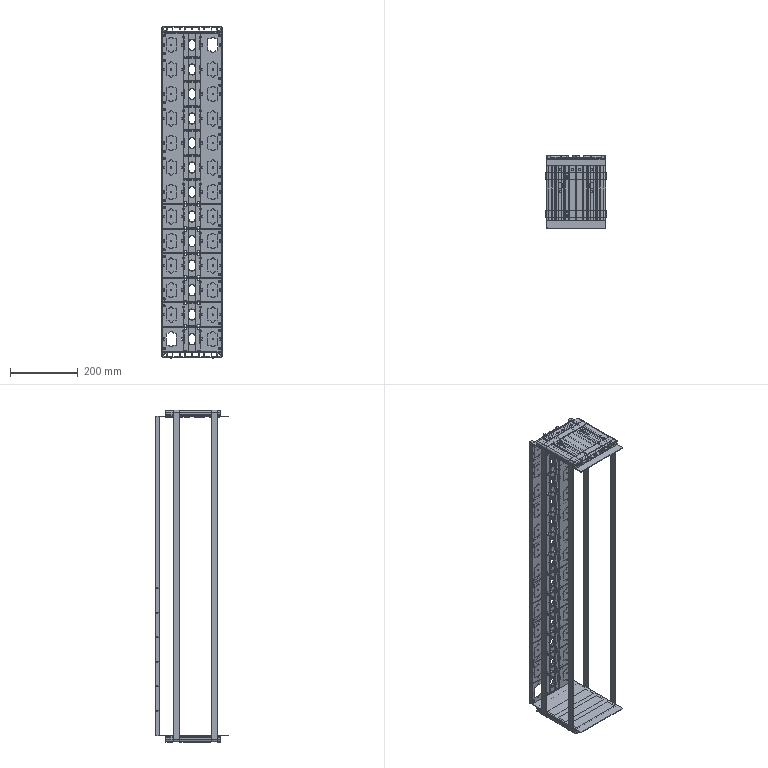Part | NX | features BREP 8 | 26 solids | 4928 faces | volume 1136806 mm3 | plane 2842 | cylinder 2086 | commonest cylinder face diameters 2 x433 4 x388 3 x204 0.6 x164 6 x128 10 x106